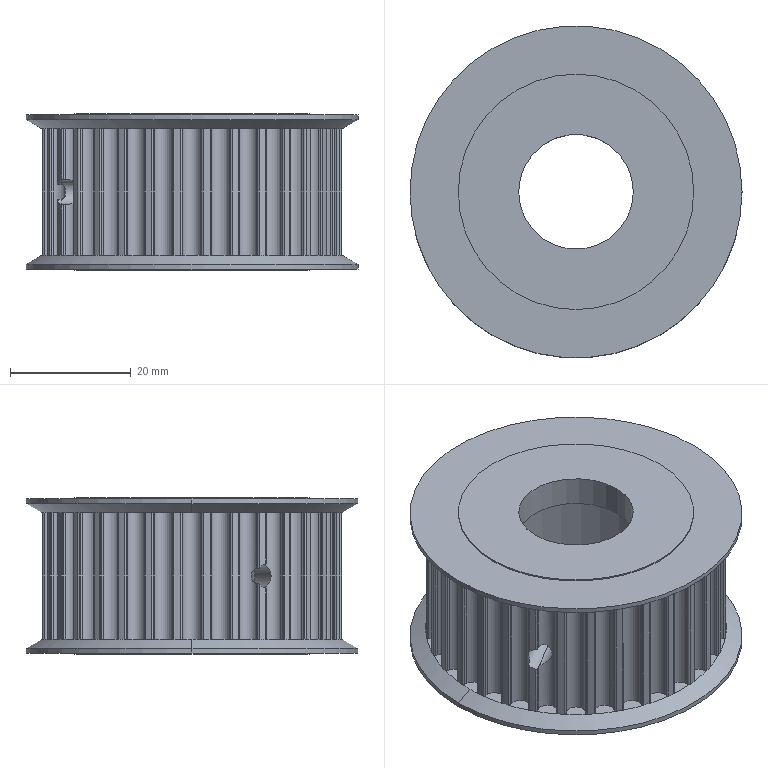Part | SolidWorks | features CirPattern 2, Cut 2, ICE 2, RefAxis 1, RevCut 1, Revolution 1 | 1 solid | 323 faces | box 55 x 55 x 26 mm | volume 25939 mm3 | cylinder 182 | plane 137 | cone 4 | commonest cylinder face diameters 0.5 x85 3.155 x48 49.79 x33 4 x4 39 x4 55 x4